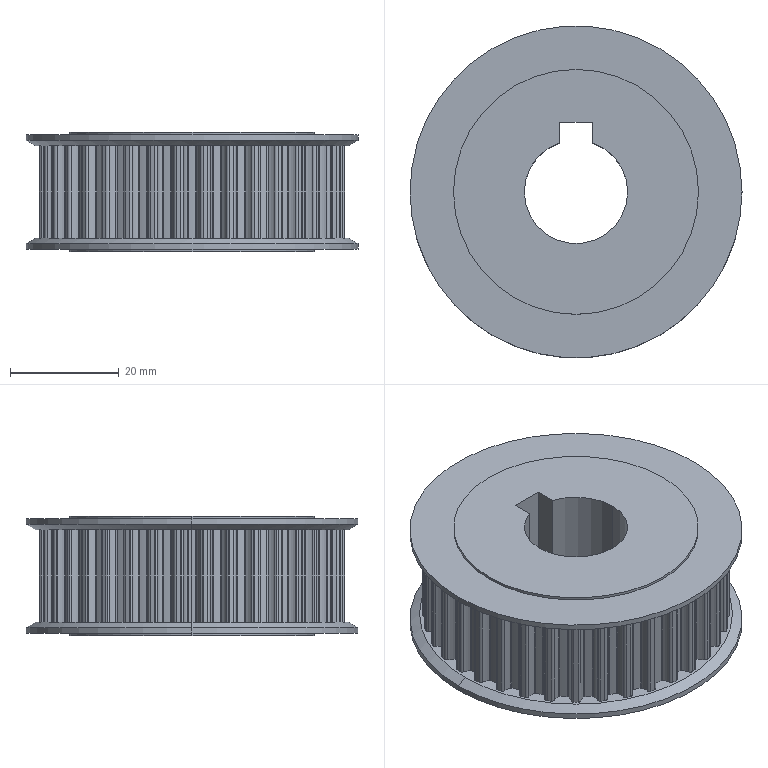Part | STEP file | Y-EAB01-S5M150-36-A-H-d28 tube-turning motor main pulley SGN-2-16 | 1 solid | 345 faces | box 61 x 61 x 22 mm | volume 45765 mm3 | cylinder 332 | plane 9 | cone 4 | commonest cylinder face diameters 1 x88 0.5 x82 6.55 x78 52.8 x37 56.34 x36 45 x4